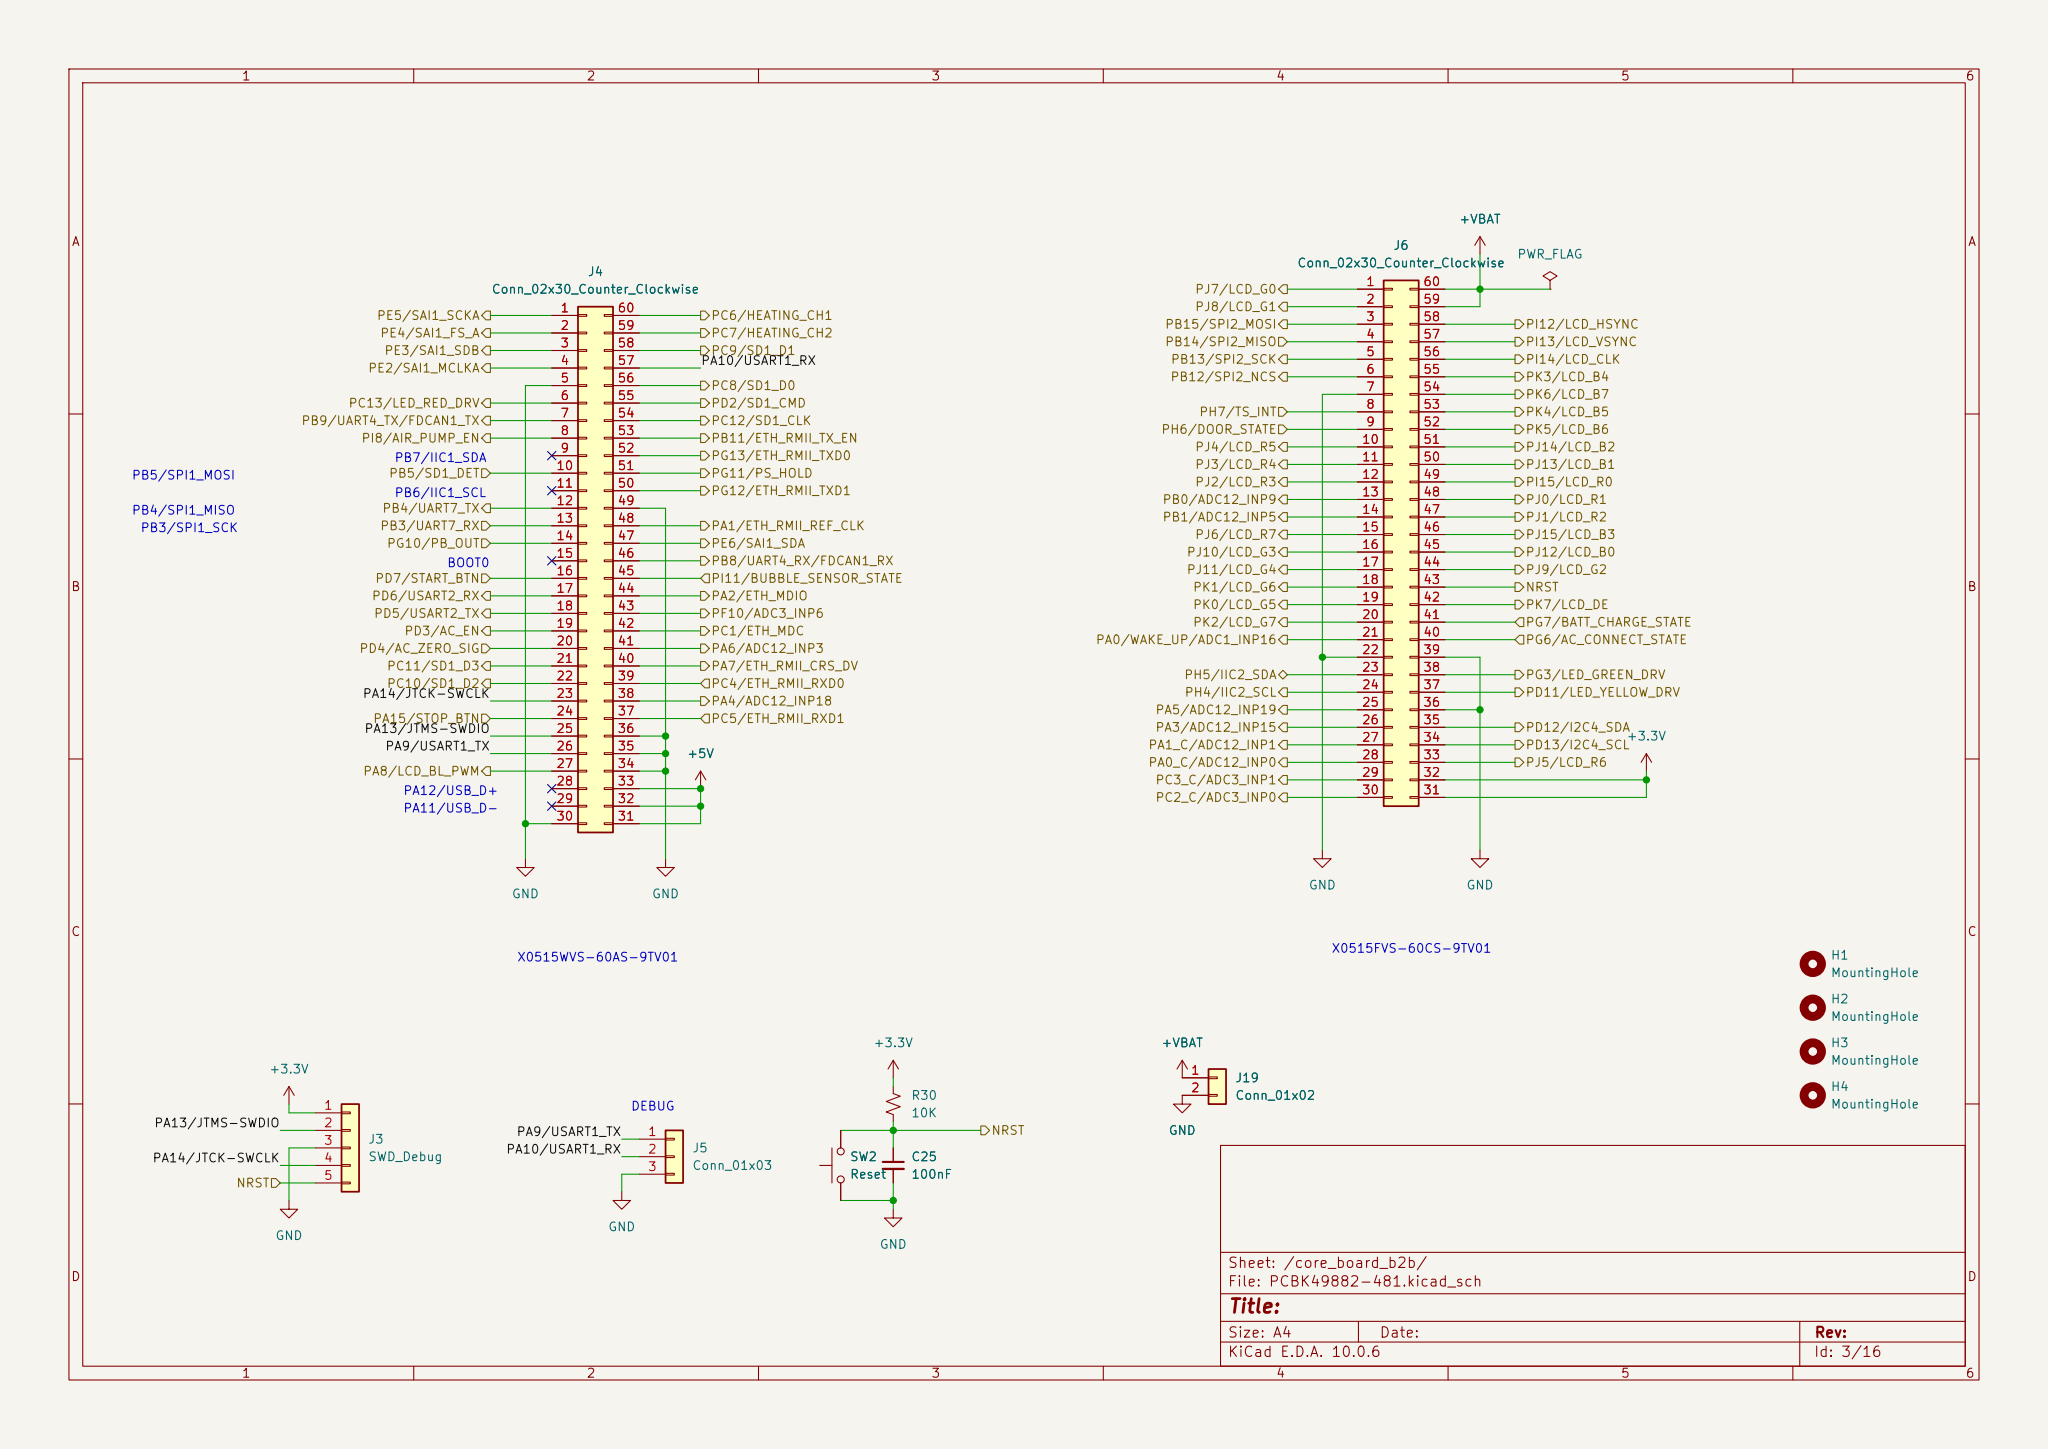Circuit board | KiCad | 536 parts | 438 nets | one sheet of the schematic
Parts on this sheet (reference | value | footprint):
C25 | 100nF | Capacitor_SMD:C_0603_1608Metric
J19
J3 | SWD_Debug | Connector_JST:JST_EH_B5B-EH-A_1x05_P2.50mm_Vertical
J4 | Conn_02x30_Counter_Clockwise | Audio_Module:Hirose_DF12_DF12C3.0-60DS-0.5V_2x30_P0.50mm_Vertical2
J6 | Conn_02x30_Counter_Clockwise | Audio_Module:Hirose_DF12_DF12C3.0-60DS-0.5V_2x30_P0.50mm_Vertical2
SW2 | Reset | Button_Switch_SMD:SW_Push_1P1T_NO_6x6mm_H9.5mm
Nets of these parts (net: part-pin ...):
+3.3V: J3-1 J6-31 J6-32
+5V: J4-31 J4-32 J4-33
+VBAT: J19-1 J6-59 J6-60
/core_board_b2b/NRST: C25-1 J3-5 SW2-2 J6-43
/core_board_b2b/PA13{slash}JTMS-SWDIO: J3-2 J4-25
/core_board_b2b/PA14{slash}JTCK-SWCLK: J3-4 J4-23
GND: C25-2 J3-3 J19-2 SW2-1 J4-5 J4-30 J4-34 J4-35 J4-36 J4-49 J6-7 J6-22 J6-36 J6-39